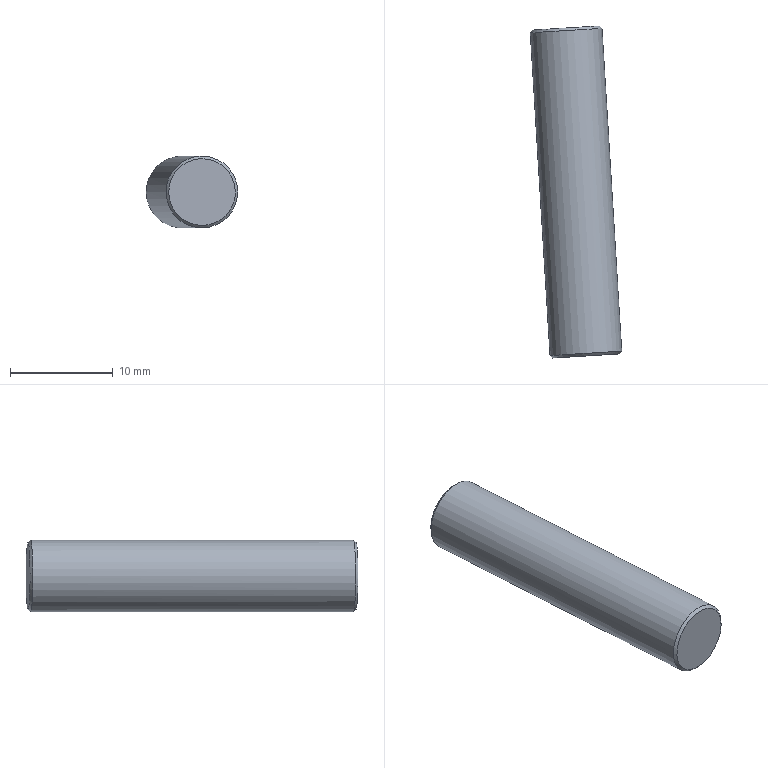Part | STEP file | 车灯-后视镜_id418_x_t | 1 solid | 5 faces | box 8.91 x 32.338 x 7 mm | volume 1230 mm3 | plane 2 | spline 2 | cylinder 1 | commonest cylinder face diameters 7 x1